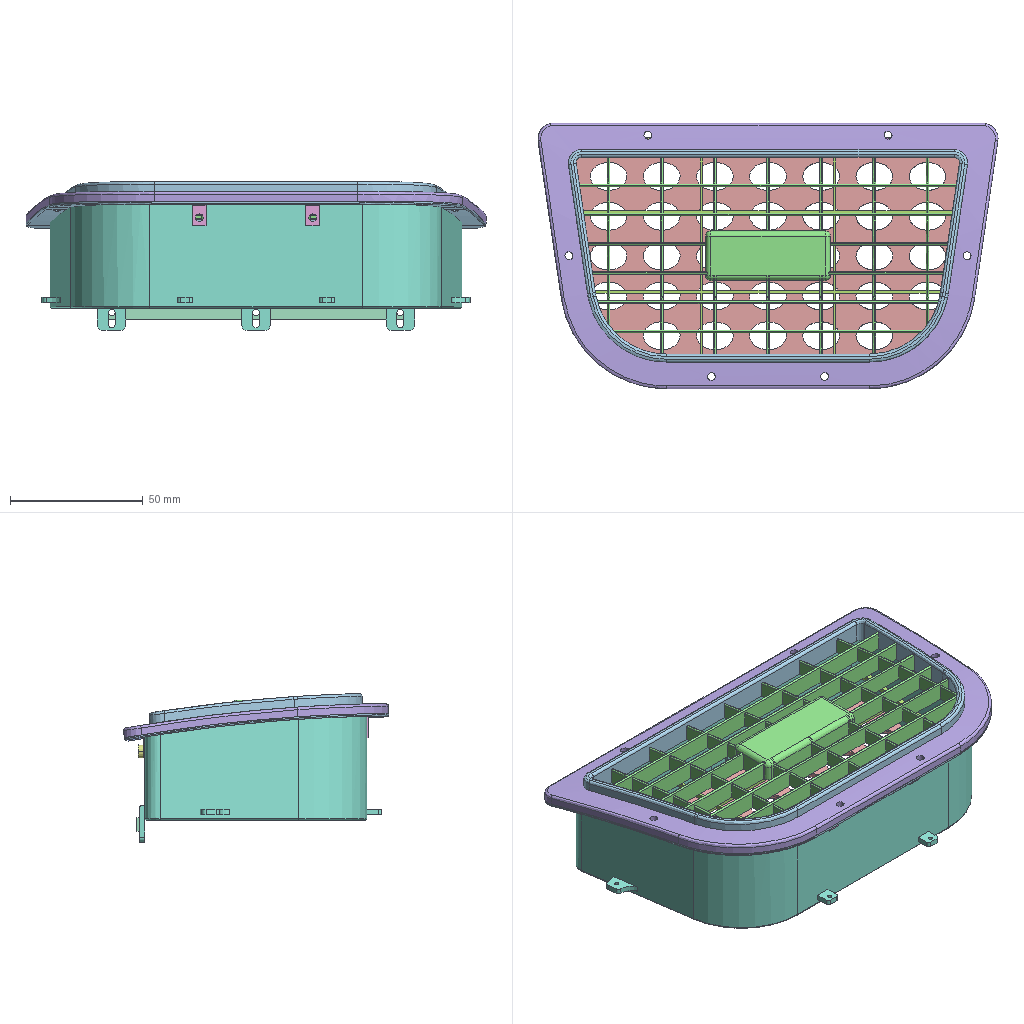Assembly | SolidWorks | 15 different items | 17 placed | box 173 x 100 x 56 mm
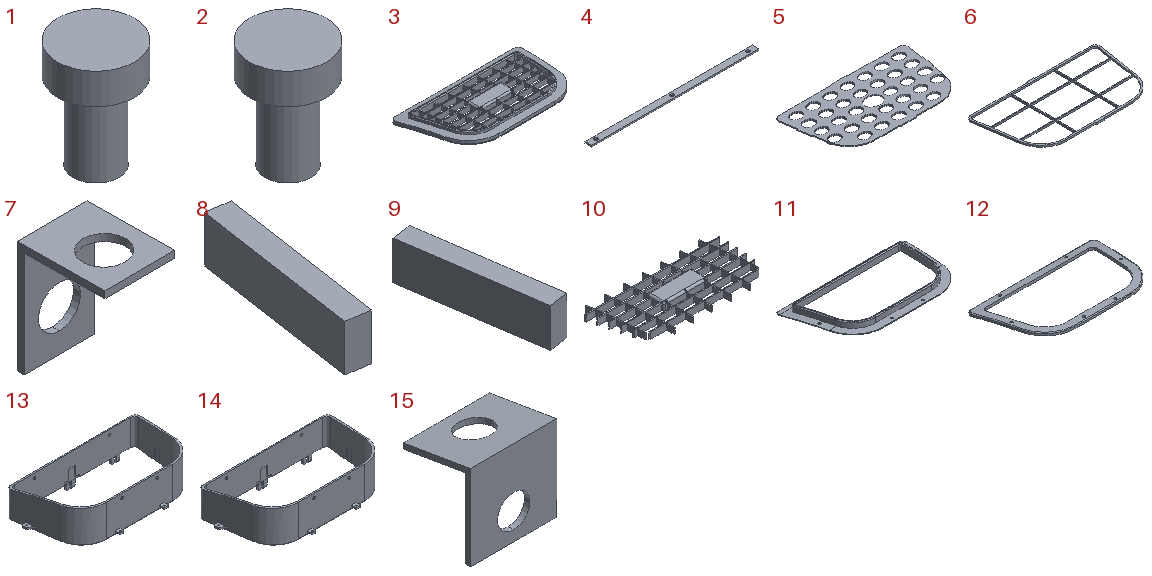Parts list (item | quantity | size | volume | features):
1 | x1 | 4.973 x 4.973 x 7 mm | 74.187 mm3 | features Extrusion 1, ICE 1
2 | x1 | 4.973 x 4.973 x 7 mm | 74.187 mm3 | features Extrusion 1, ICE 1
3 | x1 | 173.097 x 100 x 17.606 mm | 46536 mm3 | features ICE 12, Fillet 3, Extrusion 1
4 | x1 | 119.31 x 4.994 x 1 mm | 581.134 mm3 | features Cut 1, Extrusion 1
5 | x1 | 150.242 x 82 x 2 mm | 7695 mm3 | features SplitBody 1
6 | x1 | 150.242 x 82 x 2 mm | 2520 mm3 | features SplitBody 1
7 | x2 | 5 x 6.285 x 8.118 mm | 27.45 mm3 | features SplitBody 1
8 | x1 | 2.034 x 7.221 x 2 mm | 14.304 mm3 | features SplitBody 1
9 | x1 | 2.034 x 7.221 x 2 mm | 14.304 mm3 | features SplitBody 1
10 | x1 | 141.922 x 74 x 13.927 mm | 14904 mm3 | features SplitBody 1
11 | x1 | 173.097 x 99.379 x 17.536 mm | 14952 mm3 | features SplitBody 1
12 | x1 | 173.097 x 99.841 x 12.86 mm | 16352 mm3 | features SplitBody 1
13 | x1 | 161.389 x 91.111 x 47.426 mm | 30382 mm3 | features SavedExtBody 1
14 | x1 | 161.389 x 91.111 x 47.426 mm | 30382 mm3 | features SplitBody 1
15 | x2 | 8 x 6.232 x 7.883 mm | 47.269 mm3 | features SplitBody 1
Mates (type | each side: item.copy, entity, surface, feature):
Concentric | 11.1 face cylinder Base Part-Intake Net-1 | 7.1 face cylinder Base Part-Intake Net-1
Concentric | 14.1 face cylinder Base Part-Intake Net-1 | 7.1 face cylinder Base Part-Intake Net-1
Concentric | 12.1 face cylinder Base Part-Intake Net-1 | 15.1 face cylinder Base Part-Intake Net-1
Concentric | 14.1 face cylinder Base Part-Intake Net-1 | 15.1 face cylinder Base Part-Intake Net-1